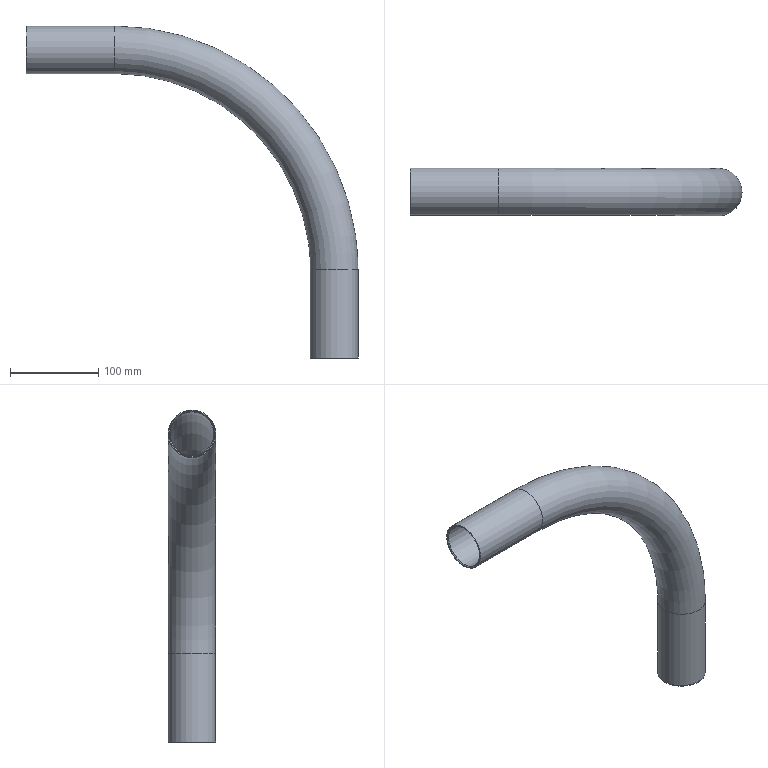Part | STEP file | JBJ-P-1007-01 | 1 solid | 10 faces | box 377 x 54 x 377 mm | volume 193491 mm3 | cylinder 4 | torus 2 | plane 2 | cone 2 | commonest cylinder face diameters 50 x2 54 x2
STEP:
#1=CARTESIAN_POINT('',(325.,0.,-349.));
#2=VERTEX_POINT('',#1);
#3=CARTESIAN_POINT('',(350.,0.,-349.));
#4=DIRECTION('',(0.,0.,-1.));
#5=DIRECTION('',(-1.,0.,0.));
#6=AXIS2_PLACEMENT_3D('',#3,#4,#5);
#7=CIRCLE('',#6,25.);
#8=EDGE_CURVE('',#2,#2,#7,.T.);
#9=ORIENTED_EDGE('',*,*,#8,.T.);
#10=EDGE_LOOP('',(#9));
#11=FACE_OUTER_BOUND('',#10,.T.);
#12=CARTESIAN_POINT('',(325.,0.,-250.));
#13=VERTEX_POINT('',#12);
#14=CARTESIAN_POINT('',(350.,0.,-250.));
#15=DIRECTION('',(0.,0.,1.));
#16=DIRECTION('',(-1.,0.,0.));
#17=AXIS2_PLACEMENT_3D('',#14,#15,#16);
#18=CIRCLE('',#17,25.);
#19=EDGE_CURVE('',#13,#13,#18,.T.);
#20=ORIENTED_EDGE('',*,*,#19,.T.);
#21=EDGE_LOOP('',(#20));
#22=FACE_OUTER_BOUND('',#21,.T.);
#23=CARTESIAN_POINT('',(350.,0.,-250.));
#24=DIRECTION('',(0.,0.,-1.));
#25=DIRECTION('',(-1.,0.,0.));
#26=AXIS2_PLACEMENT_3D('',#23,#24,#25);
#27=CYLINDRICAL_SURFACE('',#26,25.);
#28=ADVANCED_FACE('',(#11,#22),#27,.F.);
#29=ORIENTED_EDGE('',*,*,#19,.F.);
#30=EDGE_LOOP('',(#29));
#31=FACE_OUTER_BOUND('',#30,.T.);
#32=CARTESIAN_POINT('',(100.,0.,-25.));
#33=VERTEX_POINT('',#32);
#34=CARTESIAN_POINT('',(100.,0.,0.));
#35=DIRECTION('',(-1.,0.,0.));
#36=DIRECTION('',(0.,0.,-1.));
#37=AXIS2_PLACEMENT_3D('',#34,#35,#36);
#38=CIRCLE('',#37,25.);
#39=EDGE_CURVE('',#33,#33,#38,.T.);
#40=ORIENTED_EDGE('',*,*,#39,.T.);
#41=EDGE_LOOP('',(#40));
#42=FACE_OUTER_BOUND('',#41,.T.);
#43=CARTESIAN_POINT('',(100.,0.,-250.));
#44=DIRECTION('',(0.,1.,0.));
#45=DIRECTION('',(0.,0.,1.));
#46=AXIS2_PLACEMENT_3D('',#43,#44,#45);
#47=TOROIDAL_SURFACE('',#46,250.,25.);
#48=ADVANCED_FACE('',(#31,#42),#47,.F.);
#49=CARTESIAN_POINT('',(1.,0.,-25.));
#50=VERTEX_POINT('',#49);
#51=CARTESIAN_POINT('',(1.,0.,0.));
#52=DIRECTION('',(-1.,0.,0.));
#53=DIRECTION('',(0.,0.,-1.));
#54=AXIS2_PLACEMENT_3D('',#51,#52,#53);
#55=CIRCLE('',#54,25.);
#56=EDGE_CURVE('',#50,#50,#55,.T.);
#57=ORIENTED_EDGE('',*,*,#56,.T.);
#58=EDGE_LOOP('',(#57));
#59=FACE_OUTER_BOUND('',#58,.T.);
#60=ORIENTED_EDGE('',*,*,#39,.F.);
#61=EDGE_LOOP('',(#60));
#62=FACE_OUTER_BOUND('',#61,.T.);
#63=CARTESIAN_POINT('',(0.,0.,0.));
#64=DIRECTION('',(1.,0.,0.));
#65=DIRECTION('',(0.,0.,-1.));
#66=AXIS2_PLACEMENT_3D('',#63,#64,#65);
#67=CYLINDRICAL_SURFACE('',#66,25.);
#68=ADVANCED_FACE('',(#59,#62),#67,.F.);
#69=CARTESIAN_POINT('',(324.,0.,-350.));
#70=VERTEX_POINT('',#69);
#71=CARTESIAN_POINT('',(350.,0.,-350.));
#72=DIRECTION('',(0.,0.,1.));
#73=DIRECTION('',(-1.,0.,0.));
#74=AXIS2_PLACEMENT_3D('',#71,#72,#73);
#75=CIRCLE('',#74,26.);
#76=EDGE_CURVE('',#70,#70,#75,.T.);
#77=ORIENTED_EDGE('',*,*,#76,.T.);
#78=EDGE_LOOP('',(#77));
#79=FACE_BOUND('',#78,.T.);
#80=CARTESIAN_POINT('',(323.,0.,-350.));
#81=VERTEX_POINT('',#80);
#82=CARTESIAN_POINT('',(350.,0.,-350.));
#83=DIRECTION('',(0.,0.,-1.));
#84=DIRECTION('',(-1.,0.,0.));
#85=AXIS2_PLACEMENT_3D('',#82,#83,#84);
#86=CIRCLE('',#85,27.);
#87=EDGE_CURVE('',#81,#81,#86,.T.);
#88=ORIENTED_EDGE('',*,*,#87,.T.);
#89=EDGE_LOOP('',(#88));
#90=FACE_OUTER_BOUND('',#89,.T.);
#91=CARTESIAN_POINT('',(350.,0.,-350.));
#92=DIRECTION('',(0.,0.,-1.));
#93=DIRECTION('',(-1.,0.,0.));
#94=AXIS2_PLACEMENT_3D('',#91,#92,#93);
#95=PLANE('',#94);
#96=ADVANCED_FACE('',(#79,#90),#95,.T.);
#97=CARTESIAN_POINT('',(0.,0.,-26.));
#98=VERTEX_POINT('',#97);
#99=CARTESIAN_POINT('',(0.,0.,0.));
#100=DIRECTION('',(1.,0.,0.));
#101=DIRECTION('',(0.,0.,-1.));
#102=AXIS2_PLACEMENT_3D('',#99,#100,#101);
#103=CIRCLE('',#102,26.);
#104=EDGE_CURVE('',#98,#98,#103,.T.);
#105=ORIENTED_EDGE('',*,*,#104,.T.);
#106=EDGE_LOOP('',(#105));
#107=FACE_BOUND('',#106,.T.);
#108=CARTESIAN_POINT('',(0.,0.,-27.));
#109=VERTEX_POINT('',#108);
#110=CARTESIAN_POINT('',(0.,0.,0.));
#111=DIRECTION('',(1.,0.,0.));
#112=DIRECTION('',(0.,0.,-1.));
#113=AXIS2_PLACEMENT_3D('',#110,#111,#112);
#114=CIRCLE('',#113,27.);
#115=EDGE_CURVE('',#109,#109,#114,.T.);
#116=ORIENTED_EDGE('',*,*,#115,.F.);
#117=EDGE_LOOP('',(#116));
#118=FACE_OUTER_BOUND('',#117,.T.);
#119=CARTESIAN_POINT('',(0.,0.,0.));
#120=DIRECTION('',(1.,0.,0.));
#121=DIRECTION('',(0.,0.,-1.));
#122=AXIS2_PLACEMENT_3D('',#119,#120,#121);
#123=PLANE('',#122);
#124=ADVANCED_FACE('',(#107,#118),#123,.F.);
#125=ORIENTED_EDGE('',*,*,#87,.F.);
#126=EDGE_LOOP('',(#125));
#127=FACE_OUTER_BOUND('',#126,.T.);
#128=CARTESIAN_POINT('',(323.,0.,-250.));
#129=VERTEX_POINT('',#128);
#130=CARTESIAN_POINT('',(350.,0.,-250.));
#131=DIRECTION('',(0.,0.,-1.));
#132=DIRECTION('',(-1.,0.,0.));
#133=AXIS2_PLACEMENT_3D('',#130,#131,#132);
#134=CIRCLE('',#133,27.);
#135=EDGE_CURVE('',#129,#129,#134,.T.);
#136=ORIENTED_EDGE('',*,*,#135,.T.);
#137=EDGE_LOOP('',(#136));
#138=FACE_OUTER_BOUND('',#137,.T.);
#139=CARTESIAN_POINT('',(350.,0.,-250.));
#140=DIRECTION('',(0.,0.,-1.));
#141=DIRECTION('',(-1.,0.,0.));
#142=AXIS2_PLACEMENT_3D('',#139,#140,#141);
#143=CYLINDRICAL_SURFACE('',#142,27.);
#144=ADVANCED_FACE('',(#127,#138),#143,.T.);
#145=ORIENTED_EDGE('',*,*,#135,.F.);
#146=EDGE_LOOP('',(#145));
#147=FACE_OUTER_BOUND('',#146,.T.);
#148=CARTESIAN_POINT('',(100.,0.,-27.));
#149=VERTEX_POINT('',#148);
#150=CARTESIAN_POINT('',(100.,0.,0.));
#151=DIRECTION('',(1.,0.,0.));
#152=DIRECTION('',(0.,0.,-1.));
#153=AXIS2_PLACEMENT_3D('',#150,#151,#152);
#154=CIRCLE('',#153,27.);
#155=EDGE_CURVE('',#149,#149,#154,.T.);
#156=ORIENTED_EDGE('',*,*,#155,.T.);
#157=EDGE_LOOP('',(#156));
#158=FACE_OUTER_BOUND('',#157,.T.);
#159=CARTESIAN_POINT('',(100.,0.,-250.));
#160=DIRECTION('',(0.,1.,0.));
#161=DIRECTION('',(0.,0.,1.));
#162=AXIS2_PLACEMENT_3D('',#159,#160,#161);
#163=TOROIDAL_SURFACE('',#162,250.,27.);
#164=ADVANCED_FACE('',(#147,#158),#163,.T.);
#165=ORIENTED_EDGE('',*,*,#155,.F.);
#166=EDGE_LOOP('',(#165));
#167=FACE_OUTER_BOUND('',#166,.T.);
#168=ORIENTED_EDGE('',*,*,#115,.T.);
#169=EDGE_LOOP('',(#168));
#170=FACE_OUTER_BOUND('',#169,.T.);
#171=CARTESIAN_POINT('',(0.,0.,0.));
#172=DIRECTION('',(1.,0.,0.));
#173=DIRECTION('',(0.,0.,-1.));
#174=AXIS2_PLACEMENT_3D('',#171,#172,#173);
#175=CYLINDRICAL_SURFACE('',#174,27.);
#176=ADVANCED_FACE('',(#167,#170),#175,.T.);
#177=ORIENTED_EDGE('',*,*,#8,.F.);
#178=EDGE_LOOP('',(#177));
#179=FACE_BOUND('',#178,.T.);
#180=ORIENTED_EDGE('',*,*,#76,.F.);
#181=EDGE_LOOP('',(#180));
#182=FACE_OUTER_BOUND('',#181,.T.);
#183=CARTESIAN_POINT('',(350.,0.,-350.));
#184=DIRECTION('',(0.,0.,-1.));
#185=DIRECTION('',(-1.,0.,0.));
#186=AXIS2_PLACEMENT_3D('',#183,#184,#185);
#187=CONICAL_SURFACE('',#186,26.,0.7854);
#188=ADVANCED_FACE('',(#179,#182),#187,.F.);
#189=ORIENTED_EDGE('',*,*,#104,.F.);
#190=EDGE_LOOP('',(#189));
#191=FACE_OUTER_BOUND('',#190,.T.);
#192=ORIENTED_EDGE('',*,*,#56,.F.);
#193=EDGE_LOOP('',(#192));
#194=FACE_BOUND('',#193,.T.);
#195=CARTESIAN_POINT('',(1.,0.,0.));
#196=DIRECTION('',(-1.,0.,0.));
#197=DIRECTION('',(0.,0.,1.));
#198=AXIS2_PLACEMENT_3D('',#195,#196,#197);
#199=CONICAL_SURFACE('',#198,25.,0.7854);
#200=ADVANCED_FACE('',(#191,#194),#199,.F.);
#201=CLOSED_SHELL('',(#28,#48,#68,#96,#124,#144,#164,#176,#188,#200));
#202=MANIFOLD_SOLID_BREP('',#201);
#203=CARTESIAN_POINT('',(0.,0.,0.));
#204=DIRECTION('',(0.,0.,1.));
#205=DIRECTION('',(1.,0.,0.));
#206=AXIS2_PLACEMENT_3D('',#203,#204,#205);
#207=(LENGTH_UNIT()NAMED_UNIT(*)SI_UNIT(.MILLI.,.METRE.));
#208=UNCERTAINTY_MEASURE_WITH_UNIT(LENGTH_MEASURE(0.00001),#207,'','');
#209=(NAMED_UNIT(*)PLANE_ANGLE_UNIT()SI_UNIT($,.RADIAN.));
#210=(NAMED_UNIT(*)SI_UNIT($,.STERADIAN.)SOLID_ANGLE_UNIT());
#211=(GEOMETRIC_REPRESENTATION_CONTEXT(3)GLOBAL_UNCERTAINTY_ASSIGNED_CONTEXT((#208))GLOBAL_UNIT_ASSIGNED_CONTEXT((#207,#209,#210))REPRESENTATION_CONTEXT('',''));
#212=ADVANCED_BREP_SHAPE_REPRESENTATION('',(#202,#206),#211);